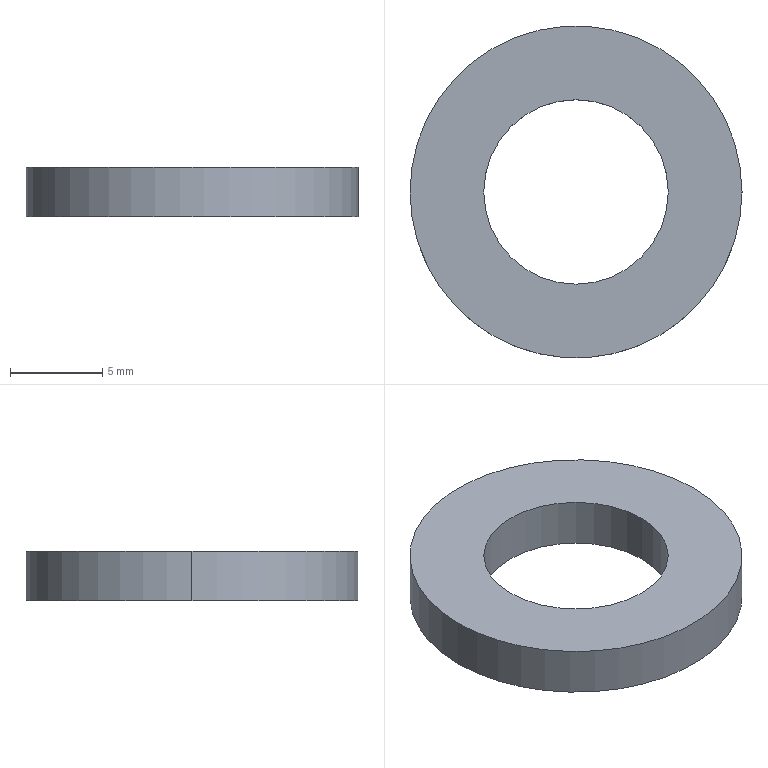Part | SolidWorks | features Extrusion 1 | 1 solid | 6 faces | box 18 x 18 x 2.7 mm | volume 475.009 mm3 | cylinder 4 | plane 2 | commonest cylinder face diameters 10 x2 18 x2
STEP:
#1=CARTESIAN_POINT('',(-5.,0.,2.7));
#2=VERTEX_POINT('',#1);
#3=CARTESIAN_POINT('',(5.,0.,2.7));
#4=VERTEX_POINT('',#3);
#5=CARTESIAN_POINT('',(0.,0.,2.7));
#6=DIRECTION('',(0.,0.,1.));
#7=DIRECTION('',(1.,0.,0.));
#8=AXIS2_PLACEMENT_3D('',#5,#6,#7);
#9=CIRCLE('',#8,5.);
#10=EDGE_CURVE('',#2,#4,#9,.T.);
#11=ORIENTED_EDGE('',*,*,#10,.T.);
#12=CARTESIAN_POINT('',(5.,0.,0.));
#13=VERTEX_POINT('',#12);
#14=CARTESIAN_POINT('',(5.,0.,2.7));
#15=DIRECTION('',(0.,0.,-1.));
#16=VECTOR('',#15,1000.);
#17=LINE('',#14,#16);
#18=EDGE_CURVE('',#4,#13,#17,.T.);
#19=ORIENTED_EDGE('',*,*,#18,.T.);
#20=CARTESIAN_POINT('',(-5.,0.,0.));
#21=VERTEX_POINT('',#20);
#22=CARTESIAN_POINT('',(0.,0.,0.));
#23=DIRECTION('',(0.,0.,1.));
#24=DIRECTION('',(1.,0.,0.));
#25=AXIS2_PLACEMENT_3D('',#22,#23,#24);
#26=CIRCLE('',#25,5.);
#27=EDGE_CURVE('',#21,#13,#26,.T.);
#28=ORIENTED_EDGE('',*,*,#27,.F.);
#29=CARTESIAN_POINT('',(-5.,0.,2.7));
#30=DIRECTION('',(0.,0.,-1.));
#31=VECTOR('',#30,1000.);
#32=LINE('',#29,#31);
#33=EDGE_CURVE('',#2,#21,#32,.T.);
#34=ORIENTED_EDGE('',*,*,#33,.F.);
#35=EDGE_LOOP('',(#11,#19,#28,#34));
#36=FACE_OUTER_BOUND('',#35,.T.);
#37=CARTESIAN_POINT('',(0.,0.,2.7));
#38=DIRECTION('',(0.,0.,-1.));
#39=DIRECTION('',(-1.,0.,0.));
#40=AXIS2_PLACEMENT_3D('',#37,#38,#39);
#41=CYLINDRICAL_SURFACE('',#40,5.);
#42=ADVANCED_FACE('',(#36),#41,.F.);
#43=CARTESIAN_POINT('',(9.,0.,2.7));
#44=VERTEX_POINT('',#43);
#45=CARTESIAN_POINT('',(-9.,0.,2.7));
#46=VERTEX_POINT('',#45);
#47=CARTESIAN_POINT('',(0.,0.,2.7));
#48=DIRECTION('',(0.,0.,1.));
#49=DIRECTION('',(1.,0.,0.));
#50=AXIS2_PLACEMENT_3D('',#47,#48,#49);
#51=CIRCLE('',#50,9.);
#52=EDGE_CURVE('',#44,#46,#51,.T.);
#53=ORIENTED_EDGE('',*,*,#52,.F.);
#54=CARTESIAN_POINT('',(9.,0.,0.));
#55=VERTEX_POINT('',#54);
#56=CARTESIAN_POINT('',(9.,0.,2.7));
#57=DIRECTION('',(0.,0.,-1.));
#58=VECTOR('',#57,1000.);
#59=LINE('',#56,#58);
#60=EDGE_CURVE('',#44,#55,#59,.T.);
#61=ORIENTED_EDGE('',*,*,#60,.T.);
#62=CARTESIAN_POINT('',(-9.,0.,0.));
#63=VERTEX_POINT('',#62);
#64=CARTESIAN_POINT('',(0.,0.,0.));
#65=DIRECTION('',(0.,0.,1.));
#66=DIRECTION('',(1.,0.,0.));
#67=AXIS2_PLACEMENT_3D('',#64,#65,#66);
#68=CIRCLE('',#67,9.);
#69=EDGE_CURVE('',#55,#63,#68,.T.);
#70=ORIENTED_EDGE('',*,*,#69,.T.);
#71=CARTESIAN_POINT('',(-9.,0.,2.7));
#72=DIRECTION('',(0.,0.,-1.));
#73=VECTOR('',#72,1000.);
#74=LINE('',#71,#73);
#75=EDGE_CURVE('',#46,#63,#74,.T.);
#76=ORIENTED_EDGE('',*,*,#75,.F.);
#77=EDGE_LOOP('',(#53,#61,#70,#76));
#78=FACE_OUTER_BOUND('',#77,.T.);
#79=CARTESIAN_POINT('',(0.,0.,2.7));
#80=DIRECTION('',(0.,0.,-1.));
#81=DIRECTION('',(-1.,0.,0.));
#82=AXIS2_PLACEMENT_3D('',#79,#80,#81);
#83=CYLINDRICAL_SURFACE('',#82,9.);
#84=ADVANCED_FACE('',(#78),#83,.T.);
#85=CARTESIAN_POINT('',(0.,0.,2.7));
#86=DIRECTION('',(0.,0.,1.));
#87=DIRECTION('',(1.,0.,0.));
#88=AXIS2_PLACEMENT_3D('',#85,#86,#87);
#89=CIRCLE('',#88,9.);
#90=EDGE_CURVE('',#46,#44,#89,.T.);
#91=ORIENTED_EDGE('',*,*,#90,.T.);
#92=ORIENTED_EDGE('',*,*,#52,.T.);
#93=EDGE_LOOP('',(#91,#92));
#94=FACE_OUTER_BOUND('',#93,.T.);
#95=ORIENTED_EDGE('',*,*,#10,.F.);
#96=CARTESIAN_POINT('',(0.,0.,2.7));
#97=DIRECTION('',(0.,0.,1.));
#98=DIRECTION('',(1.,0.,0.));
#99=AXIS2_PLACEMENT_3D('',#96,#97,#98);
#100=CIRCLE('',#99,5.);
#101=EDGE_CURVE('',#4,#2,#100,.T.);
#102=ORIENTED_EDGE('',*,*,#101,.F.);
#103=EDGE_LOOP('',(#95,#102));
#104=FACE_BOUND('',#103,.T.);
#105=CARTESIAN_POINT('',(0.,0.,2.7));
#106=DIRECTION('',(0.,0.,1.));
#107=DIRECTION('',(1.,0.,0.));
#108=AXIS2_PLACEMENT_3D('',#105,#106,#107);
#109=PLANE('',#108);
#110=ADVANCED_FACE('',(#94,#104),#109,.T.);
#111=CARTESIAN_POINT('',(0.,0.,0.));
#112=DIRECTION('',(0.,0.,1.));
#113=DIRECTION('',(1.,0.,0.));
#114=AXIS2_PLACEMENT_3D('',#111,#112,#113);
#115=CIRCLE('',#114,9.);
#116=EDGE_CURVE('',#63,#55,#115,.T.);
#117=ORIENTED_EDGE('',*,*,#116,.F.);
#118=ORIENTED_EDGE('',*,*,#69,.F.);
#119=EDGE_LOOP('',(#117,#118));
#120=FACE_OUTER_BOUND('',#119,.T.);
#121=ORIENTED_EDGE('',*,*,#27,.T.);
#122=CARTESIAN_POINT('',(0.,0.,0.));
#123=DIRECTION('',(0.,0.,1.));
#124=DIRECTION('',(1.,0.,0.));
#125=AXIS2_PLACEMENT_3D('',#122,#123,#124);
#126=CIRCLE('',#125,5.);
#127=EDGE_CURVE('',#13,#21,#126,.T.);
#128=ORIENTED_EDGE('',*,*,#127,.T.);
#129=EDGE_LOOP('',(#121,#128));
#130=FACE_BOUND('',#129,.T.);
#131=CARTESIAN_POINT('',(0.,0.,0.));
#132=DIRECTION('',(0.,0.,1.));
#133=DIRECTION('',(1.,0.,0.));
#134=AXIS2_PLACEMENT_3D('',#131,#132,#133);
#135=PLANE('',#134);
#136=ADVANCED_FACE('',(#120,#130),#135,.F.);
#137=ORIENTED_EDGE('',*,*,#60,.F.);
#138=ORIENTED_EDGE('',*,*,#90,.F.);
#139=ORIENTED_EDGE('',*,*,#75,.T.);
#140=ORIENTED_EDGE('',*,*,#116,.T.);
#141=EDGE_LOOP('',(#137,#138,#139,#140));
#142=FACE_OUTER_BOUND('',#141,.T.);
#143=CARTESIAN_POINT('',(0.,0.,2.7));
#144=DIRECTION('',(0.,0.,-1.));
#145=DIRECTION('',(-1.,0.,0.));
#146=AXIS2_PLACEMENT_3D('',#143,#144,#145);
#147=CYLINDRICAL_SURFACE('',#146,9.);
#148=ADVANCED_FACE('',(#142),#147,.T.);
#149=ORIENTED_EDGE('',*,*,#18,.F.);
#150=ORIENTED_EDGE('',*,*,#101,.T.);
#151=ORIENTED_EDGE('',*,*,#33,.T.);
#152=ORIENTED_EDGE('',*,*,#127,.F.);
#153=EDGE_LOOP('',(#149,#150,#151,#152));
#154=FACE_OUTER_BOUND('',#153,.T.);
#155=CARTESIAN_POINT('',(0.,0.,2.7));
#156=DIRECTION('',(0.,0.,-1.));
#157=DIRECTION('',(-1.,0.,0.));
#158=AXIS2_PLACEMENT_3D('',#155,#156,#157);
#159=CYLINDRICAL_SURFACE('',#158,5.);
#160=ADVANCED_FACE('',(#154),#159,.F.);
#161=CLOSED_SHELL('',(#42,#84,#110,#136,#148,#160));
#162=MANIFOLD_SOLID_BREP('',#161);
#163=CARTESIAN_POINT('',(0.,0.,0.));
#164=DIRECTION('',(0.,0.,1.));
#165=DIRECTION('',(1.,0.,0.));
#166=AXIS2_PLACEMENT_3D('',#163,#164,#165);
#167=(LENGTH_UNIT()NAMED_UNIT(*)SI_UNIT(.MILLI.,.METRE.));
#168=UNCERTAINTY_MEASURE_WITH_UNIT(LENGTH_MEASURE(0.00001),#167,'','');
#169=(NAMED_UNIT(*)PLANE_ANGLE_UNIT()SI_UNIT($,.RADIAN.));
#170=(NAMED_UNIT(*)SI_UNIT($,.STERADIAN.)SOLID_ANGLE_UNIT());
#171=(GEOMETRIC_REPRESENTATION_CONTEXT(3)GLOBAL_UNCERTAINTY_ASSIGNED_CONTEXT((#168))GLOBAL_UNIT_ASSIGNED_CONTEXT((#167,#169,#170))REPRESENTATION_CONTEXT('',''));
#172=ADVANCED_BREP_SHAPE_REPRESENTATION('',(#162,#166),#171);